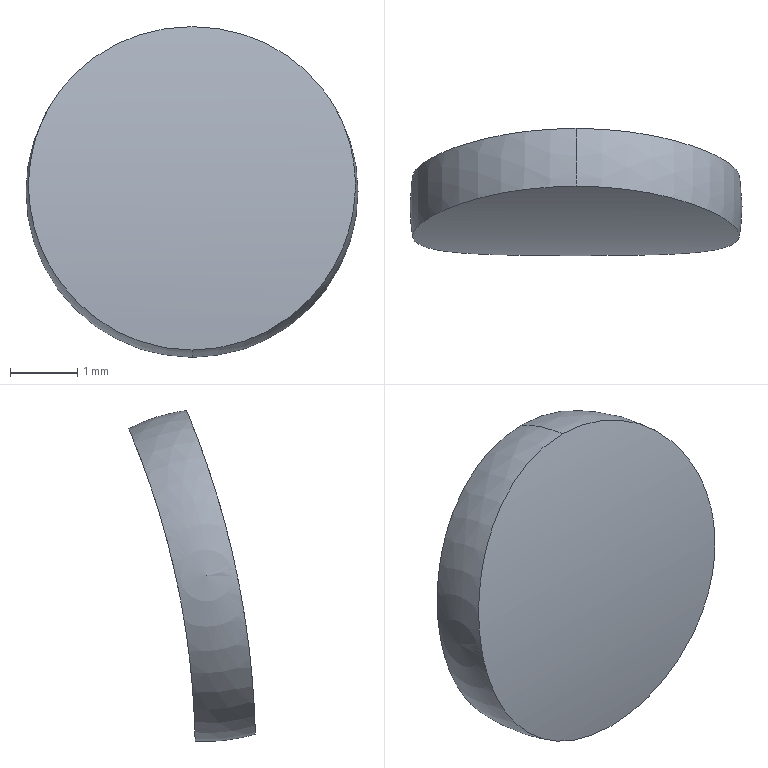Part | SolidWorks | features BaseBody 1 | 1 solid | 4 faces | box 4.95 x 1.888 x 4.932 mm | volume 17.147 mm3 | sphere 2 | cylinder 2 | commonest cylinder face diameters 25.1 x1 26.9 x1
STEP:
#1=CARTESIAN_POINT('',(0.,-13.231,0.2819));
#2=VERTEX_POINT('',#1);
#3=CARTESIAN_POINT('',(0.,-13.446,0.3379));
#4=VERTEX_POINT('',#3);
#5=CARTESIAN_POINT('',(0.,-12.716,2.703));
#6=DIRECTION('',(-1.,0.,0.));
#7=DIRECTION('',(0.,0.,1.));
#8=AXIS2_PLACEMENT_3D('',#5,#6,#7);
#9=CIRCLE('',#8,2.475);
#10=EDGE_CURVE('',#2,#4,#9,.T.);
#11=ORIENTED_EDGE('',*,*,#10,.F.);
#12=CARTESIAN_POINT('',(0.,-12.548,0.2336));
#13=VERTEX_POINT('',#12);
#14=CARTESIAN_POINT('',(0.,-12.716,2.703));
#15=DIRECTION('',(1.,0.,0.));
#16=DIRECTION('',(0.,1.,0.));
#17=AXIS2_PLACEMENT_3D('',#14,#15,#16);
#18=CIRCLE('',#17,2.475);
#19=EDGE_CURVE('',#2,#13,#18,.T.);
#20=ORIENTED_EDGE('',*,*,#19,.T.);
#21=CARTESIAN_POINT('',(0.,-11.558,4.89));
#22=VERTEX_POINT('',#21);
#23=CARTESIAN_POINT('',(0.,-11.558,4.89));
#24=CARTESIAN_POINT('',(0.1577,-11.558,4.89));
#25=CARTESIAN_POINT('',(0.3176,-11.564,4.876));
#26=CARTESIAN_POINT('',(0.6267,-11.587,4.82));
#27=CARTESIAN_POINT('',(0.7774,-11.605,4.779));
#28=CARTESIAN_POINT('',(1.071,-11.649,4.669));
#29=CARTESIAN_POINT('',(1.213,-11.677,4.6));
#30=CARTESIAN_POINT('',(1.476,-11.739,4.44));
#31=CARTESIAN_POINT('',(1.599,-11.773,4.348));
#32=CARTESIAN_POINT('',(1.827,-11.849,4.138));
#33=CARTESIAN_POINT('',(1.928,-11.888,4.024));
#34=CARTESIAN_POINT('',(2.106,-11.969,3.778));
#35=CARTESIAN_POINT('',(2.183,-12.01,3.644));
#36=CARTESIAN_POINT('',(2.307,-12.092,3.364));
#37=CARTESIAN_POINT('',(2.354,-12.131,3.22));
#38=CARTESIAN_POINT('',(2.417,-12.207,2.92));
#39=CARTESIAN_POINT('',(2.434,-12.243,2.764));
#40=CARTESIAN_POINT('',(2.434,-12.309,2.452));
#41=CARTESIAN_POINT('',(2.418,-12.339,2.298));
#42=CARTESIAN_POINT('',(2.354,-12.391,1.995));
#43=CARTESIAN_POINT('',(2.307,-12.415,1.843));
#44=CARTESIAN_POINT('',(2.183,-12.454,1.555));
#45=CARTESIAN_POINT('',(2.107,-12.47,1.418));
#46=CARTESIAN_POINT('',(1.928,-12.497,1.159));
#47=CARTESIAN_POINT('',(1.825,-12.508,1.037));
#48=CARTESIAN_POINT('',(1.487,-12.532,0.7079));
#49=CARTESIAN_POINT('',(1.216,-12.539,0.5313));
#50=CARTESIAN_POINT('',(0.7782,-12.545,0.3543));
#51=CARTESIAN_POINT('',(0.6247,-12.546,0.3088));
#52=CARTESIAN_POINT('',(0.3142,-12.548,0.2485));
#53=CARTESIAN_POINT('',(0.1577,-12.548,0.2336));
#54=CARTESIAN_POINT('',(0.,-12.548,0.2336));
#55=B_SPLINE_CURVE_WITH_KNOTS('',3,(#23,#24,#25,#26,#27,#28,#29,#30,#31,#32,#33,#34,#35,#36,#37,#38,#39,#40,#41,#42,#43,#44,#45,#46,#47,#48,#49,#50,#51,#52,#53,#54),.UNSPECIFIED.,.F.,.F.,(4,2,2,2,2,2,2,2,2,2,2,2,2,2,2,4),(0.003774,0.004246,0.004718,0.005189,0.005661,0.006132,0.006604,0.007076,0.007547,0.008019,0.008491,0.008962,0.009434,0.01038,0.01085,0.01132),.UNSPECIFIED.);
#56=EDGE_CURVE('',#22,#13,#55,.T.);
#57=ORIENTED_EDGE('',*,*,#56,.F.);
#58=CARTESIAN_POINT('',(0.,-12.201,5.124));
#59=VERTEX_POINT('',#58);
#60=CARTESIAN_POINT('',(0.,-12.716,2.703));
#61=DIRECTION('',(1.,0.,0.));
#62=DIRECTION('',(0.,1.,0.));
#63=AXIS2_PLACEMENT_3D('',#60,#61,#62);
#64=CIRCLE('',#63,2.475);
#65=EDGE_CURVE('',#22,#59,#64,.T.);
#66=ORIENTED_EDGE('',*,*,#65,.T.);
#67=CARTESIAN_POINT('',(0.,-12.421,5.16));
#68=VERTEX_POINT('',#67);
#69=CARTESIAN_POINT('',(0.,-12.716,2.703));
#70=DIRECTION('',(-1.,0.,0.));
#71=DIRECTION('',(0.,0.,1.));
#72=AXIS2_PLACEMENT_3D('',#69,#70,#71);
#73=CIRCLE('',#72,2.475);
#74=EDGE_CURVE('',#68,#59,#73,.T.);
#75=ORIENTED_EDGE('',*,*,#74,.F.);
#76=CARTESIAN_POINT('',(0.,-13.446,0.3379));
#77=CARTESIAN_POINT('',(0.1601,-13.446,0.3379));
#78=CARTESIAN_POINT('',(0.3228,-13.445,0.3544));
#79=CARTESIAN_POINT('',(0.6374,-13.444,0.419));
#80=CARTESIAN_POINT('',(0.7901,-13.442,0.4668));
#81=CARTESIAN_POINT('',(1.086,-13.437,0.593));
#82=CARTESIAN_POINT('',(1.229,-13.434,0.6716));
#83=CARTESIAN_POINT('',(1.493,-13.423,0.8527));
#84=CARTESIAN_POINT('',(1.616,-13.416,0.9564));
#85=CARTESIAN_POINT('',(1.842,-13.398,1.188));
#86=CARTESIAN_POINT('',(1.941,-13.386,1.313));
#87=CARTESIAN_POINT('',(2.116,-13.358,1.579));
#88=CARTESIAN_POINT('',(2.191,-13.34,1.723));
#89=CARTESIAN_POINT('',(2.312,-13.299,2.018));
#90=CARTESIAN_POINT('',(2.357,-13.275,2.17));
#91=CARTESIAN_POINT('',(2.418,-13.22,2.481));
#92=CARTESIAN_POINT('',(2.434,-13.189,2.64));
#93=CARTESIAN_POINT('',(2.434,-13.122,2.957));
#94=CARTESIAN_POINT('',(2.418,-13.086,3.113));
#95=CARTESIAN_POINT('',(2.357,-13.01,3.417));
#96=CARTESIAN_POINT('',(2.311,-12.969,3.568));
#97=CARTESIAN_POINT('',(2.19,-12.887,3.855));
#98=CARTESIAN_POINT('',(2.116,-12.845,3.991));
#99=CARTESIAN_POINT('',(1.941,-12.763,4.247));
#100=CARTESIAN_POINT('',(1.839,-12.722,4.367));
#101=CARTESIAN_POINT('',(1.615,-12.645,4.584));
#102=CARTESIAN_POINT('',(1.493,-12.61,4.681));
#103=CARTESIAN_POINT('',(1.227,-12.545,4.852));
#104=CARTESIAN_POINT('',(1.085,-12.516,4.924));
#105=CARTESIAN_POINT('',(0.6433,-12.447,5.099));
#106=CARTESIAN_POINT('',(0.3203,-12.421,5.16));
#107=CARTESIAN_POINT('',(0.,-12.421,5.16));
#108=B_SPLINE_CURVE_WITH_KNOTS('',3,(#76,#77,#78,#79,#80,#81,#82,#83,#84,#85,#86,#87,#88,#89,#90,#91,#92,#93,#94,#95,#96,#97,#98,#99,#100,#101,#102,#103,#104,#105,#106,#107),.UNSPECIFIED.,.F.,.F.,(4,2,2,2,2,2,2,2,2,2,2,2,2,2,2,4),(0.01152,0.012,0.01248,0.01295,0.01343,0.01391,0.01439,0.01487,0.01535,0.01583,0.01631,0.01679,0.01727,0.01775,0.01823,0.01919),.UNSPECIFIED.);
#109=EDGE_CURVE('',#4,#68,#108,.T.);
#110=ORIENTED_EDGE('',*,*,#109,.F.);
#111=EDGE_LOOP('',(#11,#20,#57,#66,#75,#110));
#112=FACE_OUTER_BOUND('',#111,.T.);
#113=CARTESIAN_POINT('',(0.,-12.716,2.703));
#114=DIRECTION('',(1.,0.,0.));
#115=DIRECTION('',(0.,-0.9781,0.2079));
#116=AXIS2_PLACEMENT_3D('',#113,#114,#115);
#117=SPHERICAL_SURFACE('',#116,2.475);
#118=ADVANCED_FACE('',(#112),#117,.T.);
#119=ORIENTED_EDGE('',*,*,#56,.T.);
#120=CARTESIAN_POINT('',(0.,-12.548,0.2336));
#121=CARTESIAN_POINT('',(-0.1577,-12.548,0.2336));
#122=CARTESIAN_POINT('',(-0.3176,-12.548,0.249));
#123=CARTESIAN_POINT('',(-0.6267,-12.546,0.3093));
#124=CARTESIAN_POINT('',(-0.7775,-12.545,0.354));
#125=CARTESIAN_POINT('',(-1.071,-12.541,0.4729));
#126=CARTESIAN_POINT('',(-1.213,-12.538,0.5469));
#127=CARTESIAN_POINT('',(-1.476,-12.53,0.7185));
#128=CARTESIAN_POINT('',(-1.599,-12.524,0.8169));
#129=CARTESIAN_POINT('',(-1.827,-12.507,1.039));
#130=CARTESIAN_POINT('',(-1.928,-12.497,1.159));
#131=CARTESIAN_POINT('',(-2.106,-12.47,1.417));
#132=CARTESIAN_POINT('',(-2.183,-12.454,1.556));
#133=CARTESIAN_POINT('',(-2.307,-12.415,1.845));
#134=CARTESIAN_POINT('',(-2.354,-12.392,1.993));
#135=CARTESIAN_POINT('',(-2.417,-12.339,2.298));
#136=CARTESIAN_POINT('',(-2.434,-12.309,2.454));
#137=CARTESIAN_POINT('',(-2.434,-12.242,2.766));
#138=CARTESIAN_POINT('',(-2.418,-12.207,2.919));
#139=CARTESIAN_POINT('',(-2.354,-12.131,3.218));
#140=CARTESIAN_POINT('',(-2.307,-12.091,3.366));
#141=CARTESIAN_POINT('',(-2.183,-12.01,3.645));
#142=CARTESIAN_POINT('',(-2.107,-11.969,3.777));
#143=CARTESIAN_POINT('',(-1.928,-11.888,4.025));
#144=CARTESIAN_POINT('',(-1.825,-11.848,4.14));
#145=CARTESIAN_POINT('',(-1.487,-11.736,4.45));
#146=CARTESIAN_POINT('',(-1.216,-11.671,4.615));
#147=CARTESIAN_POINT('',(-0.7782,-11.605,4.779));
#148=CARTESIAN_POINT('',(-0.6247,-11.587,4.821));
#149=CARTESIAN_POINT('',(-0.3142,-11.564,4.876));
#150=CARTESIAN_POINT('',(-0.1577,-11.558,4.89));
#151=CARTESIAN_POINT('',(0.,-11.558,4.89));
#152=B_SPLINE_CURVE_WITH_KNOTS('',3,(#120,#121,#122,#123,#124,#125,#126,#127,#128,#129,#130,#131,#132,#133,#134,#135,#136,#137,#138,#139,#140,#141,#142,#143,#144,#145,#146,#147,#148,#149,#150,#151),.UNSPECIFIED.,.F.,.F.,(4,2,2,2,2,2,2,2,2,2,2,2,2,2,2,4),(0.01132,0.01179,0.01226,0.01274,0.01321,0.01368,0.01415,0.01462,0.01509,0.01557,0.01604,0.01651,0.01698,0.01792,0.0184,0.01887),.UNSPECIFIED.);
#153=EDGE_CURVE('',#13,#22,#152,.T.);
#154=ORIENTED_EDGE('',*,*,#153,.T.);
#155=EDGE_LOOP('',(#119,#154));
#156=FACE_OUTER_BOUND('',#155,.T.);
#157=CARTESIAN_POINT('',(-19.927,0.,0.));
#158=DIRECTION('',(-1.,0.,0.));
#159=DIRECTION('',(0.,0.,1.));
#160=AXIS2_PLACEMENT_3D('',#157,#158,#159);
#161=CYLINDRICAL_SURFACE('',#160,12.55);
#162=ADVANCED_FACE('',(#156),#161,.F.);
#163=CARTESIAN_POINT('',(0.,-12.421,5.16));
#164=CARTESIAN_POINT('',(-0.1601,-12.421,5.16));
#165=CARTESIAN_POINT('',(-0.3228,-12.427,5.145));
#166=CARTESIAN_POINT('',(-0.6374,-12.452,5.085));
#167=CARTESIAN_POINT('',(-0.7901,-12.47,5.041));
#168=CARTESIAN_POINT('',(-1.086,-12.517,4.924));
#169=CARTESIAN_POINT('',(-1.229,-12.545,4.85));
#170=CARTESIAN_POINT('',(-1.493,-12.61,4.681));
#171=CARTESIAN_POINT('',(-1.616,-12.646,4.583));
#172=CARTESIAN_POINT('',(-1.842,-12.723,4.364));
#173=CARTESIAN_POINT('',(-1.941,-12.763,4.246));
#174=CARTESIAN_POINT('',(-2.116,-12.845,3.99));
#175=CARTESIAN_POINT('',(-2.191,-12.888,3.852));
#176=CARTESIAN_POINT('',(-2.312,-12.97,3.565));
#177=CARTESIAN_POINT('',(-2.357,-13.01,3.417));
#178=CARTESIAN_POINT('',(-2.418,-13.086,3.111));
#179=CARTESIAN_POINT('',(-2.434,-13.123,2.953));
#180=CARTESIAN_POINT('',(-2.434,-13.19,2.635));
#181=CARTESIAN_POINT('',(-2.418,-13.221,2.479));
#182=CARTESIAN_POINT('',(-2.357,-13.275,2.17));
#183=CARTESIAN_POINT('',(-2.311,-13.299,2.015));
#184=CARTESIAN_POINT('',(-2.19,-13.34,1.72));
#185=CARTESIAN_POINT('',(-2.116,-13.358,1.579));
#186=CARTESIAN_POINT('',(-1.941,-13.387,1.312));
#187=CARTESIAN_POINT('',(-1.839,-13.398,1.184));
#188=CARTESIAN_POINT('',(-1.615,-13.416,0.9557));
#189=CARTESIAN_POINT('',(-1.493,-13.423,0.8527));
#190=CARTESIAN_POINT('',(-1.227,-13.434,0.6703));
#191=CARTESIAN_POINT('',(-1.085,-13.437,0.5922));
#192=CARTESIAN_POINT('',(-0.6433,-13.445,0.4043));
#193=CARTESIAN_POINT('',(-0.3203,-13.446,0.3379));
#194=CARTESIAN_POINT('',(0.,-13.446,0.3379));
#195=B_SPLINE_CURVE_WITH_KNOTS('',3,(#163,#164,#165,#166,#167,#168,#169,#170,#171,#172,#173,#174,#175,#176,#177,#178,#179,#180,#181,#182,#183,#184,#185,#186,#187,#188,#189,#190,#191,#192,#193,#194),.UNSPECIFIED.,.F.,.F.,(4,2,2,2,2,2,2,2,2,2,2,2,2,2,2,4),(0.00384,0.00432,0.0048,0.005279,0.005759,0.006239,0.006719,0.007198,0.007678,0.008158,0.008637,0.009117,0.009597,0.01008,0.01056,0.01152),.UNSPECIFIED.);
#196=EDGE_CURVE('',#68,#4,#195,.T.);
#197=ORIENTED_EDGE('',*,*,#196,.T.);
#198=ORIENTED_EDGE('',*,*,#109,.T.);
#199=EDGE_LOOP('',(#197,#198));
#200=FACE_OUTER_BOUND('',#199,.T.);
#201=CARTESIAN_POINT('',(-19.927,0.,0.));
#202=DIRECTION('',(-1.,0.,0.));
#203=DIRECTION('',(0.,0.,1.));
#204=AXIS2_PLACEMENT_3D('',#201,#202,#203);
#205=CYLINDRICAL_SURFACE('',#204,13.45);
#206=ADVANCED_FACE('',(#200),#205,.T.);
#207=ORIENTED_EDGE('',*,*,#19,.F.);
#208=ORIENTED_EDGE('',*,*,#10,.T.);
#209=ORIENTED_EDGE('',*,*,#196,.F.);
#210=ORIENTED_EDGE('',*,*,#74,.T.);
#211=ORIENTED_EDGE('',*,*,#65,.F.);
#212=ORIENTED_EDGE('',*,*,#153,.F.);
#213=EDGE_LOOP('',(#207,#208,#209,#210,#211,#212));
#214=FACE_OUTER_BOUND('',#213,.T.);
#215=CARTESIAN_POINT('',(0.,-12.716,2.703));
#216=DIRECTION('',(1.,0.,0.));
#217=DIRECTION('',(0.,-0.9781,0.2079));
#218=AXIS2_PLACEMENT_3D('',#215,#216,#217);
#219=SPHERICAL_SURFACE('',#218,2.475);
#220=ADVANCED_FACE('',(#214),#219,.T.);
#221=CLOSED_SHELL('',(#118,#162,#206,#220));
#222=MANIFOLD_SOLID_BREP('',#221);
#223=CARTESIAN_POINT('',(0.,0.,0.));
#224=DIRECTION('',(0.,0.,1.));
#225=DIRECTION('',(1.,0.,0.));
#226=AXIS2_PLACEMENT_3D('',#223,#224,#225);
#227=(LENGTH_UNIT()NAMED_UNIT(*)SI_UNIT(.MILLI.,.METRE.));
#228=UNCERTAINTY_MEASURE_WITH_UNIT(LENGTH_MEASURE(0.00001),#227,'','');
#229=(NAMED_UNIT(*)PLANE_ANGLE_UNIT()SI_UNIT($,.RADIAN.));
#230=(NAMED_UNIT(*)SI_UNIT($,.STERADIAN.)SOLID_ANGLE_UNIT());
#231=(GEOMETRIC_REPRESENTATION_CONTEXT(3)GLOBAL_UNCERTAINTY_ASSIGNED_CONTEXT((#228))GLOBAL_UNIT_ASSIGNED_CONTEXT((#227,#229,#230))REPRESENTATION_CONTEXT('',''));
#232=ADVANCED_BREP_SHAPE_REPRESENTATION('',(#222,#226),#231);